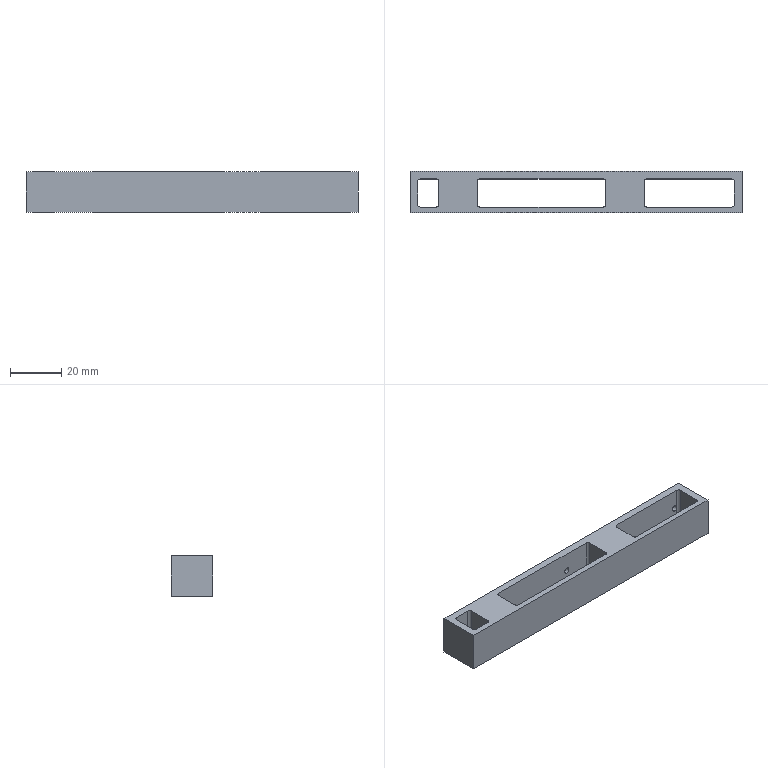NC program | NX | posted with a generic post | part box 130 x 16.2 x 16 mm
Lines 19504 to 19599 of 19599:
(PLANAR_MILL , TOOL : D6A45)
N38976 T07 M6
N38978 G54
N38980 G17 G0 G90 X43.585 Y-4.643 B0. C0. S9500 M3
N38982 G43 Z30. H7
N38984 Z0.5
N38986 G94 G1 Z-1. F1250.
N38988 G3 X44.351 Y-5. R1.
N38990 G1 X61.
N38992 X61.065 Y-5.013
N38994 X61.113 Y-4.965
N38996 X61.1 Y-4.9
N38998 Y4.1
N39000 X61.113 Y4.165
N39002 X61.065 Y4.213
N39004 X61. Y4.2
N39006 X27.702
N39008 X27.637 Y4.213
N39010 X27.589 Y4.165
N39012 X27.602 Y4.1
N39014 Y-4.9
N39016 X27.589 Y-4.965
N39018 X27.637 Y-5.013
N39020 X27.702 Y-5.
N39022 X44.351
N39024 G3 X45.117 Y-4.643 R1.
N39026 G1 Z0.5
N39028 G0 Z30.
N39030 X-0.766 Y9.357
N39032 Z0.5
N39034 G1 Z-1.
N39036 G3 X0. Y9. R1.
N39038 G1 X65.
N39040 G2 X65.9 Y8.1 R0.9
N39042 G1 Y-8.1
N39044 G2 X65. Y-9. R0.9
N39046 G1 X-65.
N39048 G2 X-65.9 Y-8.1 R0.9
N39050 G1 Y8.1
N39052 G2 X-65. Y9. R0.9
N39054 G1 X0.
N39056 G3 X0.766 Y9.357 R1.
N39058 G1 Z0.5
N39060 G0 Z30.
N39062 X-12.737 Y3.843
N39064 Z0.5
N39066 G1 Z-1.
N39068 G3 X-13.503 Y4.2 R1.
N39070 G1 X-37.708
N39072 X-37.773 Y4.213
N39074 X-37.821 Y4.165
N39076 X-37.808 Y4.1
N39078 Y-4.9
N39080 X-37.821 Y-4.965
N39082 X-37.773 Y-5.013
N39084 X-37.708 Y-5.
N39086 X10.702
N39088 X10.767 Y-5.013
N39090 X10.814 Y-4.965
N39092 X10.802 Y-4.9
N39094 Y4.1
N39096 X10.814 Y4.165
N39098 X10.767 Y4.213
N39100 X10.702 Y4.2
N39102 X-13.503
N39104 G3 X-14.269 Y3.843 R1.
N39106 G1 Z0.5
N39108 G0 Z30.
N39110 X-60.743 Y0.366
N39112 Z0.5
N39114 G1 Z-1.
N39116 G3 X-61.1 Y-0.4 R1.
N39118 G1 Y-4.9
N39120 X-61.113 Y-4.965
N39122 X-61.065 Y-5.013
N39124 X-61. Y-5.
N39126 X-54.708
N39128 X-54.643 Y-5.013
N39130 X-54.596 Y-4.965
N39132 X-54.608 Y-4.9
N39134 Y4.1
N39136 X-54.596 Y4.165
N39138 X-54.643 Y4.213
N39140 X-54.708 Y4.2
N39142 X-61.
N39144 X-61.065 Y4.213
N39146 X-61.113 Y4.165
N39148 X-61.1 Y4.1
N39150 Y-0.4
N39152 G3 X-60.743 Y-1.166 R1.
N39154 G1 Z0.5
N39156 G0 Z30.
N39158 M5
N39160 M2